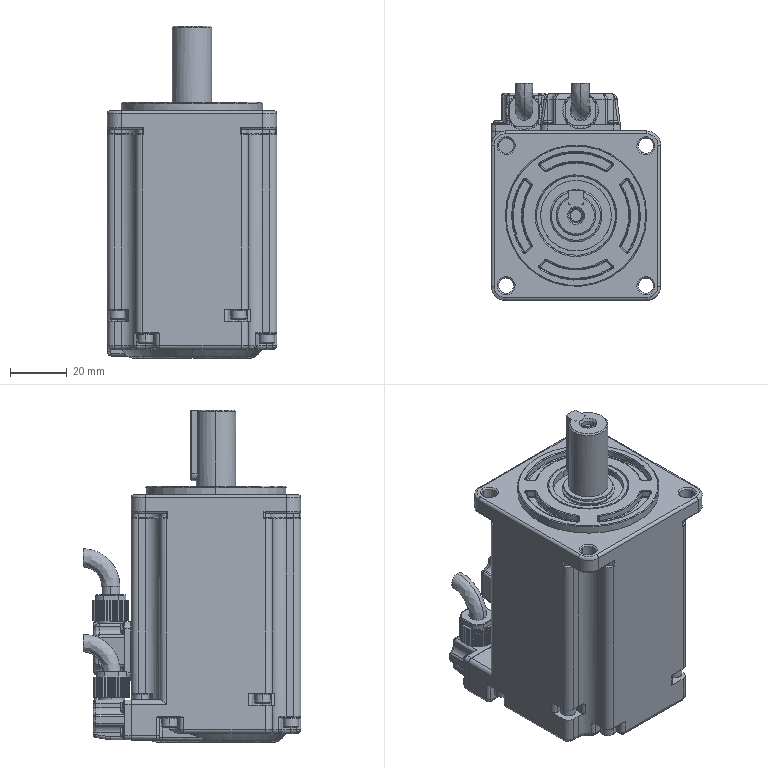Part | STEP file | Heqi 400W motor X2MH040A-N2L (wire type) | 1 solid | 1514 faces | box 60 x 76.95 x 117.5 mm | volume 299796 mm3 | cylinder 552 | plane 526 | spline 248 | cone 100 | torus 59 | other 29 | commonest cylinder face diameters 0.2 x192 5 x44 3 x33 1.1 x32 4.2 x26 2 x25